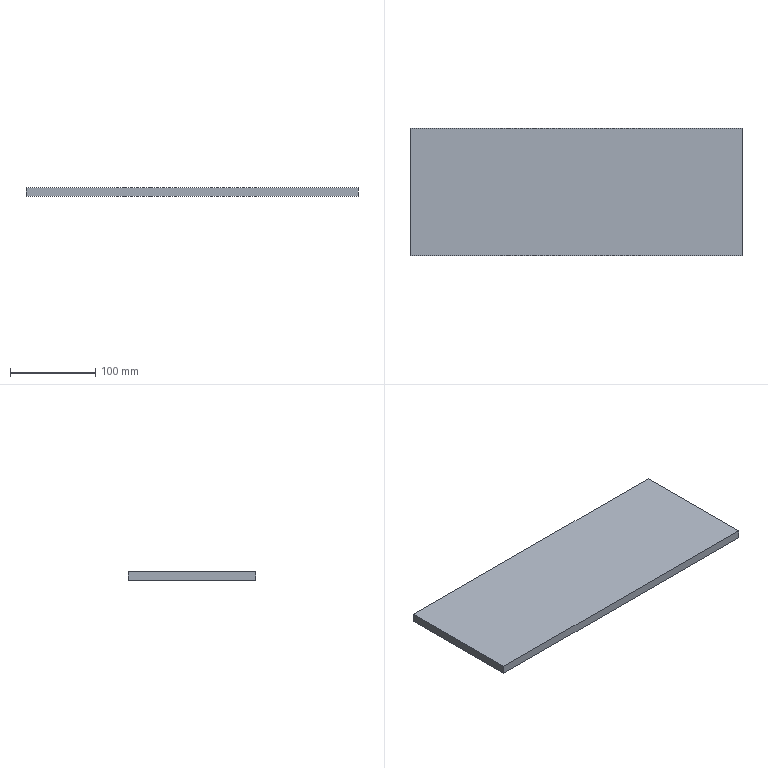Part | NX | features BREP 1 | 1 solid | 6 faces | box 390 x 150 x 10 mm | volume 585000 mm3 | plane 6
STEP:
#1=CARTESIAN_POINT('',(-195.,75.,-5.));
#2=VERTEX_POINT('',#1);
#3=CARTESIAN_POINT('',(-195.,-75.,-5.));
#4=VERTEX_POINT('',#3);
#5=CARTESIAN_POINT('',(-195.,75.,-5.));
#6=DIRECTION('',(0.,-1.,0.));
#7=VECTOR('',#6,1000.);
#8=LINE('',#5,#7);
#9=EDGE_CURVE('',#2,#4,#8,.T.);
#10=ORIENTED_EDGE('',*,*,#9,.T.);
#11=CARTESIAN_POINT('',(-195.,-75.,5.));
#12=VERTEX_POINT('',#11);
#13=CARTESIAN_POINT('',(-195.,-75.,5.));
#14=DIRECTION('',(0.,0.,-1.));
#15=VECTOR('',#14,1000.);
#16=LINE('',#13,#15);
#17=EDGE_CURVE('',#12,#4,#16,.T.);
#18=ORIENTED_EDGE('',*,*,#17,.F.);
#19=CARTESIAN_POINT('',(-195.,75.,5.));
#20=VERTEX_POINT('',#19);
#21=CARTESIAN_POINT('',(-195.,75.,5.));
#22=DIRECTION('',(0.,-1.,0.));
#23=VECTOR('',#22,1000.);
#24=LINE('',#21,#23);
#25=EDGE_CURVE('',#20,#12,#24,.T.);
#26=ORIENTED_EDGE('',*,*,#25,.F.);
#27=CARTESIAN_POINT('',(-195.,75.,5.));
#28=DIRECTION('',(0.,0.,-1.));
#29=VECTOR('',#28,1000.);
#30=LINE('',#27,#29);
#31=EDGE_CURVE('',#20,#2,#30,.T.);
#32=ORIENTED_EDGE('',*,*,#31,.T.);
#33=EDGE_LOOP('',(#10,#18,#26,#32));
#34=FACE_BOUND('',#33,.T.);
#35=CARTESIAN_POINT('',(-195.,75.,5.));
#36=DIRECTION('',(1.,0.,0.));
#37=DIRECTION('',(0.,0.,1.));
#38=AXIS2_PLACEMENT_3D('',#35,#36,#37);
#39=PLANE('',#38);
#40=ADVANCED_FACE('',(#34),#39,.F.);
#41=CARTESIAN_POINT('',(195.,-75.,-5.));
#42=VERTEX_POINT('',#41);
#43=CARTESIAN_POINT('',(-195.,-75.,-5.));
#44=DIRECTION('',(1.,0.,0.));
#45=VECTOR('',#44,1000.);
#46=LINE('',#43,#45);
#47=EDGE_CURVE('',#4,#42,#46,.T.);
#48=ORIENTED_EDGE('',*,*,#47,.T.);
#49=CARTESIAN_POINT('',(195.,-75.,5.));
#50=VERTEX_POINT('',#49);
#51=CARTESIAN_POINT('',(195.,-75.,5.));
#52=DIRECTION('',(0.,0.,-1.));
#53=VECTOR('',#52,1000.);
#54=LINE('',#51,#53);
#55=EDGE_CURVE('',#50,#42,#54,.T.);
#56=ORIENTED_EDGE('',*,*,#55,.F.);
#57=CARTESIAN_POINT('',(-195.,-75.,5.));
#58=DIRECTION('',(1.,0.,0.));
#59=VECTOR('',#58,1000.);
#60=LINE('',#57,#59);
#61=EDGE_CURVE('',#12,#50,#60,.T.);
#62=ORIENTED_EDGE('',*,*,#61,.F.);
#63=ORIENTED_EDGE('',*,*,#17,.T.);
#64=EDGE_LOOP('',(#48,#56,#62,#63));
#65=FACE_BOUND('',#64,.T.);
#66=CARTESIAN_POINT('',(-195.,-75.,5.));
#67=DIRECTION('',(0.,1.,0.));
#68=DIRECTION('',(0.,0.,-1.));
#69=AXIS2_PLACEMENT_3D('',#66,#67,#68);
#70=PLANE('',#69);
#71=ADVANCED_FACE('',(#65),#70,.F.);
#72=CARTESIAN_POINT('',(195.,75.,-5.));
#73=VERTEX_POINT('',#72);
#74=CARTESIAN_POINT('',(195.,75.,-5.));
#75=DIRECTION('',(0.,1.,0.));
#76=VECTOR('',#75,1000.);
#77=LINE('',#74,#76);
#78=EDGE_CURVE('',#42,#73,#77,.T.);
#79=ORIENTED_EDGE('',*,*,#78,.T.);
#80=CARTESIAN_POINT('',(195.,75.,5.));
#81=VERTEX_POINT('',#80);
#82=CARTESIAN_POINT('',(195.,75.,5.));
#83=DIRECTION('',(0.,0.,-1.));
#84=VECTOR('',#83,1000.);
#85=LINE('',#82,#84);
#86=EDGE_CURVE('',#81,#73,#85,.T.);
#87=ORIENTED_EDGE('',*,*,#86,.F.);
#88=CARTESIAN_POINT('',(195.,75.,5.));
#89=DIRECTION('',(0.,1.,0.));
#90=VECTOR('',#89,1000.);
#91=LINE('',#88,#90);
#92=EDGE_CURVE('',#50,#81,#91,.T.);
#93=ORIENTED_EDGE('',*,*,#92,.F.);
#94=ORIENTED_EDGE('',*,*,#55,.T.);
#95=EDGE_LOOP('',(#79,#87,#93,#94));
#96=FACE_BOUND('',#95,.T.);
#97=CARTESIAN_POINT('',(195.,75.,5.));
#98=DIRECTION('',(-1.,0.,0.));
#99=DIRECTION('',(0.,0.,-1.));
#100=AXIS2_PLACEMENT_3D('',#97,#98,#99);
#101=PLANE('',#100);
#102=ADVANCED_FACE('',(#96),#101,.F.);
#103=CARTESIAN_POINT('',(-195.,75.,-5.));
#104=DIRECTION('',(-1.,0.,0.));
#105=VECTOR('',#104,1000.);
#106=LINE('',#103,#105);
#107=EDGE_CURVE('',#73,#2,#106,.T.);
#108=ORIENTED_EDGE('',*,*,#107,.T.);
#109=ORIENTED_EDGE('',*,*,#31,.F.);
#110=CARTESIAN_POINT('',(-195.,75.,5.));
#111=DIRECTION('',(-1.,0.,0.));
#112=VECTOR('',#111,1000.);
#113=LINE('',#110,#112);
#114=EDGE_CURVE('',#81,#20,#113,.T.);
#115=ORIENTED_EDGE('',*,*,#114,.F.);
#116=ORIENTED_EDGE('',*,*,#86,.T.);
#117=EDGE_LOOP('',(#108,#109,#115,#116));
#118=FACE_BOUND('',#117,.T.);
#119=CARTESIAN_POINT('',(-195.,75.,5.));
#120=DIRECTION('',(0.,-1.,0.));
#121=DIRECTION('',(0.,0.,1.));
#122=AXIS2_PLACEMENT_3D('',#119,#120,#121);
#123=PLANE('',#122);
#124=ADVANCED_FACE('',(#118),#123,.F.);
#125=ORIENTED_EDGE('',*,*,#25,.T.);
#126=ORIENTED_EDGE('',*,*,#61,.T.);
#127=ORIENTED_EDGE('',*,*,#92,.T.);
#128=ORIENTED_EDGE('',*,*,#114,.T.);
#129=EDGE_LOOP('',(#125,#126,#127,#128));
#130=FACE_BOUND('',#129,.T.);
#131=CARTESIAN_POINT('',(-195.,-75.,5.));
#132=DIRECTION('',(0.,0.,1.));
#133=DIRECTION('',(-1.,0.,0.));
#134=AXIS2_PLACEMENT_3D('',#131,#132,#133);
#135=PLANE('',#134);
#136=ADVANCED_FACE('',(#130),#135,.T.);
#137=ORIENTED_EDGE('',*,*,#9,.F.);
#138=ORIENTED_EDGE('',*,*,#107,.F.);
#139=ORIENTED_EDGE('',*,*,#78,.F.);
#140=ORIENTED_EDGE('',*,*,#47,.F.);
#141=EDGE_LOOP('',(#137,#138,#139,#140));
#142=FACE_BOUND('',#141,.T.);
#143=CARTESIAN_POINT('',(-195.,-75.,-5.));
#144=DIRECTION('',(0.,0.,1.));
#145=DIRECTION('',(-1.,0.,0.));
#146=AXIS2_PLACEMENT_3D('',#143,#144,#145);
#147=PLANE('',#146);
#148=ADVANCED_FACE('',(#142),#147,.F.);
#149=CLOSED_SHELL('',(#40,#71,#102,#124,#136,#148));
#150=MANIFOLD_SOLID_BREP('',#149);
#151=(LENGTH_UNIT()NAMED_UNIT(*)SI_UNIT(.MILLI.,.METRE.));
#152=UNCERTAINTY_MEASURE_WITH_UNIT(LENGTH_MEASURE(0.00001),#151,'','');
#153=(NAMED_UNIT(*)PLANE_ANGLE_UNIT()SI_UNIT($,.RADIAN.));
#154=(NAMED_UNIT(*)SI_UNIT($,.STERADIAN.)SOLID_ANGLE_UNIT());
#155=(GEOMETRIC_REPRESENTATION_CONTEXT(3)GLOBAL_UNCERTAINTY_ASSIGNED_CONTEXT((#152))GLOBAL_UNIT_ASSIGNED_CONTEXT((#151,#153,#154))REPRESENTATION_CONTEXT('',''));
#156=ADVANCED_BREP_SHAPE_REPRESENTATION('',(#150),#155);